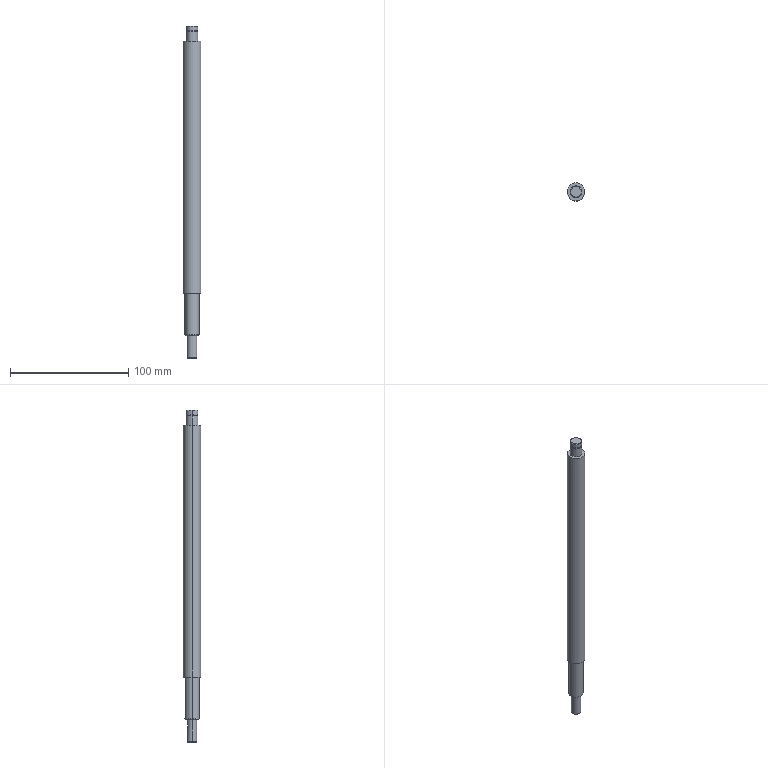Part | SolidWorks | features RevCut 4, Chamfer 2, Extrusion 1, ICE 1 | 1 solid | 28 faces | box 15 x 15 x 281 mm | volume 43646 mm3 | cylinder 12 | plane 9 | cone 7 | commonest cylinder face diameters 10 x4 8 x2 9.5 x2 12 x2 15 x2
STEP:
#1=CARTESIAN_POINT('',(4.5,0.,281.));
#2=VERTEX_POINT('',#1);
#3=CARTESIAN_POINT('',(-4.5,0.,281.));
#4=VERTEX_POINT('',#3);
#5=CARTESIAN_POINT('',(0.,0.,281.));
#6=DIRECTION('',(0.,0.,1.));
#7=DIRECTION('',(1.,0.,0.));
#8=AXIS2_PLACEMENT_3D('',#5,#6,#7);
#9=CIRCLE('',#8,4.5);
#10=EDGE_CURVE('',#2,#4,#9,.T.);
#11=ORIENTED_EDGE('',*,*,#10,.F.);
#12=CARTESIAN_POINT('',(5.,0.,280.5));
#13=VERTEX_POINT('',#12);
#14=CARTESIAN_POINT('',(4.5,0.,281.));
#15=DIRECTION('',(0.7071,0.,-0.7071));
#16=VECTOR('',#15,1000.);
#17=LINE('',#14,#16);
#18=EDGE_CURVE('',#2,#13,#17,.T.);
#19=ORIENTED_EDGE('',*,*,#18,.T.);
#20=CARTESIAN_POINT('',(-5.,0.,280.5));
#21=VERTEX_POINT('',#20);
#22=CARTESIAN_POINT('',(0.,0.,280.5));
#23=DIRECTION('',(0.,0.,-1.));
#24=DIRECTION('',(1.,0.,0.));
#25=AXIS2_PLACEMENT_3D('',#22,#23,#24);
#26=CIRCLE('',#25,5.);
#27=EDGE_CURVE('',#21,#13,#26,.T.);
#28=ORIENTED_EDGE('',*,*,#27,.F.);
#29=CARTESIAN_POINT('',(-4.5,0.,281.));
#30=DIRECTION('',(-0.7071,0.,-0.7071));
#31=VECTOR('',#30,1000.);
#32=LINE('',#29,#31);
#33=EDGE_CURVE('',#4,#21,#32,.T.);
#34=ORIENTED_EDGE('',*,*,#33,.F.);
#35=EDGE_LOOP('',(#11,#19,#28,#34));
#36=FACE_OUTER_BOUND('',#35,.T.);
#37=CARTESIAN_POINT('',(0.,0.,281.));
#38=DIRECTION('',(0.,0.,-1.));
#39=DIRECTION('',(-1.,0.,0.));
#40=AXIS2_PLACEMENT_3D('',#37,#38,#39);
#41=CONICAL_SURFACE('',#40,4.5,0.7854);
#42=ADVANCED_FACE('',(#36),#41,.T.);
#43=CARTESIAN_POINT('',(-5.,0.,277.1));
#44=VERTEX_POINT('',#43);
#45=CARTESIAN_POINT('',(5.,0.,277.1));
#46=VERTEX_POINT('',#45);
#47=CARTESIAN_POINT('',(0.,0.,277.1));
#48=DIRECTION('',(0.,0.,-1.));
#49=DIRECTION('',(1.,0.,0.));
#50=AXIS2_PLACEMENT_3D('',#47,#48,#49);
#51=CIRCLE('',#50,5.);
#52=EDGE_CURVE('',#44,#46,#51,.T.);
#53=ORIENTED_EDGE('',*,*,#52,.F.);
#54=CARTESIAN_POINT('',(-5.,0.,281.));
#55=DIRECTION('',(0.,0.,1.));
#56=VECTOR('',#55,1000.);
#57=LINE('',#54,#56);
#58=EDGE_CURVE('',#44,#21,#57,.T.);
#59=ORIENTED_EDGE('',*,*,#58,.T.);
#60=ORIENTED_EDGE('',*,*,#27,.T.);
#61=CARTESIAN_POINT('',(5.,0.,281.));
#62=DIRECTION('',(0.,0.,1.));
#63=VECTOR('',#62,1000.);
#64=LINE('',#61,#63);
#65=EDGE_CURVE('',#46,#13,#64,.T.);
#66=ORIENTED_EDGE('',*,*,#65,.F.);
#67=EDGE_LOOP('',(#53,#59,#60,#66));
#68=FACE_OUTER_BOUND('',#67,.T.);
#69=CARTESIAN_POINT('',(0.,0.,281.));
#70=DIRECTION('',(0.,0.,1.));
#71=DIRECTION('',(1.,0.,0.));
#72=AXIS2_PLACEMENT_3D('',#69,#70,#71);
#73=CYLINDRICAL_SURFACE('',#72,5.);
#74=ADVANCED_FACE('',(#68),#73,.T.);
#75=CARTESIAN_POINT('',(-4.75,0.,277.1));
#76=VERTEX_POINT('',#75);
#77=CARTESIAN_POINT('',(4.75,0.,277.1));
#78=VERTEX_POINT('',#77);
#79=CARTESIAN_POINT('',(0.,0.,277.1));
#80=DIRECTION('',(0.,0.,-1.));
#81=DIRECTION('',(-1.,0.,0.));
#82=AXIS2_PLACEMENT_3D('',#79,#80,#81);
#83=CIRCLE('',#82,4.75);
#84=EDGE_CURVE('',#76,#78,#83,.T.);
#85=ORIENTED_EDGE('',*,*,#84,.T.);
#86=CARTESIAN_POINT('',(4.75,0.,276.));
#87=VERTEX_POINT('',#86);
#88=CARTESIAN_POINT('',(4.75,0.,268.));
#89=DIRECTION('',(0.,0.,-1.));
#90=VECTOR('',#89,1000.);
#91=LINE('',#88,#90);
#92=EDGE_CURVE('',#78,#87,#91,.T.);
#93=ORIENTED_EDGE('',*,*,#92,.T.);
#94=CARTESIAN_POINT('',(-4.75,0.,276.));
#95=VERTEX_POINT('',#94);
#96=CARTESIAN_POINT('',(0.,0.,276.));
#97=DIRECTION('',(0.,0.,-1.));
#98=DIRECTION('',(-1.,0.,0.));
#99=AXIS2_PLACEMENT_3D('',#96,#97,#98);
#100=CIRCLE('',#99,4.75);
#101=EDGE_CURVE('',#95,#87,#100,.T.);
#102=ORIENTED_EDGE('',*,*,#101,.F.);
#103=CARTESIAN_POINT('',(-4.75,0.,268.));
#104=DIRECTION('',(0.,0.,-1.));
#105=VECTOR('',#104,1000.);
#106=LINE('',#103,#105);
#107=EDGE_CURVE('',#76,#95,#106,.T.);
#108=ORIENTED_EDGE('',*,*,#107,.F.);
#109=EDGE_LOOP('',(#85,#93,#102,#108));
#110=FACE_OUTER_BOUND('',#109,.T.);
#111=CARTESIAN_POINT('',(0.,0.,268.));
#112=DIRECTION('',(0.,0.,-1.));
#113=DIRECTION('',(-1.,0.,0.));
#114=AXIS2_PLACEMENT_3D('',#111,#112,#113);
#115=CYLINDRICAL_SURFACE('',#114,4.75);
#116=ADVANCED_FACE('',(#110),#115,.T.);
#117=CARTESIAN_POINT('',(-5.5,0.,19.));
#118=VERTEX_POINT('',#117);
#119=CARTESIAN_POINT('',(5.5,0.,19.));
#120=VERTEX_POINT('',#119);
#121=CARTESIAN_POINT('',(0.,0.,19.));
#122=DIRECTION('',(0.,0.,-1.));
#123=DIRECTION('',(1.,0.,0.));
#124=AXIS2_PLACEMENT_3D('',#121,#122,#123);
#125=CIRCLE('',#124,5.5);
#126=EDGE_CURVE('',#118,#120,#125,.T.);
#127=ORIENTED_EDGE('',*,*,#126,.F.);
#128=CARTESIAN_POINT('',(-6.,0.,19.5));
#129=VERTEX_POINT('',#128);
#130=CARTESIAN_POINT('',(-6.,0.,19.5));
#131=DIRECTION('',(-0.7071,0.,0.7071));
#132=VECTOR('',#131,1000.);
#133=LINE('',#130,#132);
#134=EDGE_CURVE('',#118,#129,#133,.T.);
#135=ORIENTED_EDGE('',*,*,#134,.T.);
#136=CARTESIAN_POINT('',(6.,0.,19.5));
#137=VERTEX_POINT('',#136);
#138=CARTESIAN_POINT('',(0.,0.,19.5));
#139=DIRECTION('',(0.,0.,1.));
#140=DIRECTION('',(1.,0.,0.));
#141=AXIS2_PLACEMENT_3D('',#138,#139,#140);
#142=CIRCLE('',#141,6.);
#143=EDGE_CURVE('',#137,#129,#142,.T.);
#144=ORIENTED_EDGE('',*,*,#143,.F.);
#145=CARTESIAN_POINT('',(6.,0.,19.5));
#146=DIRECTION('',(0.7071,0.,0.7071));
#147=VECTOR('',#146,1000.);
#148=LINE('',#145,#147);
#149=EDGE_CURVE('',#120,#137,#148,.T.);
#150=ORIENTED_EDGE('',*,*,#149,.F.);
#151=EDGE_LOOP('',(#127,#135,#144,#150));
#152=FACE_OUTER_BOUND('',#151,.T.);
#153=CARTESIAN_POINT('',(0.,0.,19.5));
#154=DIRECTION('',(0.,0.,1.));
#155=DIRECTION('',(1.,0.,0.));
#156=AXIS2_PLACEMENT_3D('',#153,#154,#155);
#157=CONICAL_SURFACE('',#156,6.,0.7854);
#158=ADVANCED_FACE('',(#152),#157,.T.);
#159=CARTESIAN_POINT('',(-3.5,0.,0.));
#160=VERTEX_POINT('',#159);
#161=CARTESIAN_POINT('',(0.,3.5,0.));
#162=VERTEX_POINT('',#161);
#163=CARTESIAN_POINT('',(0.,0.,0.));
#164=DIRECTION('',(0.,0.,-1.));
#165=DIRECTION('',(1.,0.,0.));
#166=AXIS2_PLACEMENT_3D('',#163,#164,#165);
#167=CIRCLE('',#166,3.5);
#168=EDGE_CURVE('',#160,#162,#167,.T.);
#169=ORIENTED_EDGE('',*,*,#168,.F.);
#170=CARTESIAN_POINT('',(-4.,0.,0.5));
#171=VERTEX_POINT('',#170);
#172=CARTESIAN_POINT('',(-3.5,0.,0.));
#173=DIRECTION('',(-0.7071,0.,0.7071));
#174=VECTOR('',#173,1000.);
#175=LINE('',#172,#174);
#176=EDGE_CURVE('',#160,#171,#175,.T.);
#177=ORIENTED_EDGE('',*,*,#176,.T.);
#178=CARTESIAN_POINT('',(-1.936,3.5,0.5));
#179=VERTEX_POINT('',#178);
#180=CARTESIAN_POINT('',(0.,0.,0.5));
#181=DIRECTION('',(0.,0.,1.));
#182=DIRECTION('',(1.,0.,0.));
#183=AXIS2_PLACEMENT_3D('',#180,#181,#182);
#184=CIRCLE('',#183,4.);
#185=EDGE_CURVE('',#179,#171,#184,.T.);
#186=ORIENTED_EDGE('',*,*,#185,.F.);
#187=CARTESIAN_POINT('',(0.,3.5,0.));
#188=CARTESIAN_POINT('',(-0.34,3.5,0.));
#189=CARTESIAN_POINT('',(-0.673,3.5,0.05018));
#190=CARTESIAN_POINT('',(-1.328,3.5,0.2302));
#191=CARTESIAN_POINT('',(-1.638,3.5,0.3555));
#192=CARTESIAN_POINT('',(-1.936,3.5,0.5));
#193=B_SPLINE_CURVE_WITH_KNOTS('',3,(#187,#188,#189,#190,#191,#192),.UNSPECIFIED.,.F.,.F.,(4,2,4),(0.004182,0.005183,0.006184),.UNSPECIFIED.);
#194=EDGE_CURVE('',#162,#179,#193,.T.);
#195=ORIENTED_EDGE('',*,*,#194,.F.);
#196=EDGE_LOOP('',(#169,#177,#186,#195));
#197=FACE_OUTER_BOUND('',#196,.T.);
#198=CARTESIAN_POINT('',(0.,0.,0.));
#199=DIRECTION('',(0.,0.,1.));
#200=DIRECTION('',(1.,0.,0.));
#201=AXIS2_PLACEMENT_3D('',#198,#199,#200);
#202=CONICAL_SURFACE('',#201,3.5,0.7854);
#203=ADVANCED_FACE('',(#197),#202,.T.);
#204=ORIENTED_EDGE('',*,*,#176,.F.);
#205=CARTESIAN_POINT('',(3.5,0.,0.));
#206=VERTEX_POINT('',#205);
#207=CARTESIAN_POINT('',(0.,0.,0.));
#208=DIRECTION('',(0.,0.,-1.));
#209=DIRECTION('',(1.,0.,0.));
#210=AXIS2_PLACEMENT_3D('',#207,#208,#209);
#211=CIRCLE('',#210,3.5);
#212=EDGE_CURVE('',#206,#160,#211,.T.);
#213=ORIENTED_EDGE('',*,*,#212,.F.);
#214=CARTESIAN_POINT('',(4.,0.,0.5));
#215=VERTEX_POINT('',#214);
#216=CARTESIAN_POINT('',(3.5,0.,0.));
#217=DIRECTION('',(0.7071,0.,0.7071));
#218=VECTOR('',#217,1000.);
#219=LINE('',#216,#218);
#220=EDGE_CURVE('',#206,#215,#219,.T.);
#221=ORIENTED_EDGE('',*,*,#220,.T.);
#222=CARTESIAN_POINT('',(0.,0.,0.5));
#223=DIRECTION('',(0.,0.,1.));
#224=DIRECTION('',(1.,0.,0.));
#225=AXIS2_PLACEMENT_3D('',#222,#223,#224);
#226=CIRCLE('',#225,4.);
#227=EDGE_CURVE('',#171,#215,#226,.T.);
#228=ORIENTED_EDGE('',*,*,#227,.F.);
#229=EDGE_LOOP('',(#204,#213,#221,#228));
#230=FACE_OUTER_BOUND('',#229,.T.);
#231=CARTESIAN_POINT('',(0.,0.,0.));
#232=DIRECTION('',(0.,0.,1.));
#233=DIRECTION('',(1.,0.,0.));
#234=AXIS2_PLACEMENT_3D('',#231,#232,#233);
#235=CONICAL_SURFACE('',#234,3.5,0.7854);
#236=ADVANCED_FACE('',(#230),#235,.T.);
#237=CARTESIAN_POINT('',(-4.,0.,19.));
#238=VERTEX_POINT('',#237);
#239=CARTESIAN_POINT('',(4.,0.,19.));
#240=VERTEX_POINT('',#239);
#241=CARTESIAN_POINT('',(0.,0.,19.));
#242=DIRECTION('',(0.,0.,-1.));
#243=DIRECTION('',(-1.,0.,0.));
#244=AXIS2_PLACEMENT_3D('',#241,#242,#243);
#245=CIRCLE('',#244,4.);
#246=EDGE_CURVE('',#238,#240,#245,.T.);
#247=ORIENTED_EDGE('',*,*,#246,.T.);
#248=CARTESIAN_POINT('',(4.,0.,0.));
#249=DIRECTION('',(0.,0.,-1.));
#250=VECTOR('',#249,1000.);
#251=LINE('',#248,#250);
#252=EDGE_CURVE('',#240,#215,#251,.T.);
#253=ORIENTED_EDGE('',*,*,#252,.T.);
#254=CARTESIAN_POINT('',(1.936,3.5,0.5));
#255=VERTEX_POINT('',#254);
#256=CARTESIAN_POINT('',(0.,0.,0.5));
#257=DIRECTION('',(0.,0.,1.));
#258=DIRECTION('',(1.,0.,0.));
#259=AXIS2_PLACEMENT_3D('',#256,#257,#258);
#260=CIRCLE('',#259,4.);
#261=EDGE_CURVE('',#215,#255,#260,.T.);
#262=ORIENTED_EDGE('',*,*,#261,.T.);
#263=CARTESIAN_POINT('',(1.936,3.5,17.));
#264=VERTEX_POINT('',#263);
#265=CARTESIAN_POINT('',(1.936,3.5,0.));
#266=DIRECTION('',(0.,0.,1.));
#267=VECTOR('',#266,1000.);
#268=LINE('',#265,#267);
#269=EDGE_CURVE('',#255,#264,#268,.T.);
#270=ORIENTED_EDGE('',*,*,#269,.T.);
#271=CARTESIAN_POINT('',(-1.936,3.5,17.));
#272=VERTEX_POINT('',#271);
#273=CARTESIAN_POINT('',(0.,0.,17.));
#274=DIRECTION('',(0.,0.,-1.));
#275=DIRECTION('',(-1.,0.,0.));
#276=AXIS2_PLACEMENT_3D('',#273,#274,#275);
#277=CIRCLE('',#276,4.);
#278=EDGE_CURVE('',#272,#264,#277,.T.);
#279=ORIENTED_EDGE('',*,*,#278,.F.);
#280=CARTESIAN_POINT('',(-1.936,3.5,0.));
#281=DIRECTION('',(0.,0.,-1.));
#282=VECTOR('',#281,1000.);
#283=LINE('',#280,#282);
#284=EDGE_CURVE('',#272,#179,#283,.T.);
#285=ORIENTED_EDGE('',*,*,#284,.T.);
#286=ORIENTED_EDGE('',*,*,#185,.T.);
#287=CARTESIAN_POINT('',(-4.,0.,0.));
#288=DIRECTION('',(0.,0.,-1.));
#289=VECTOR('',#288,1000.);
#290=LINE('',#287,#289);
#291=EDGE_CURVE('',#238,#171,#290,.T.);
#292=ORIENTED_EDGE('',*,*,#291,.F.);
#293=EDGE_LOOP('',(#247,#253,#262,#270,#279,#285,#286,#292));
#294=FACE_OUTER_BOUND('',#293,.T.);
#295=CARTESIAN_POINT('',(0.,0.,0.));
#296=DIRECTION('',(0.,0.,-1.));
#297=DIRECTION('',(-1.,0.,0.));
#298=AXIS2_PLACEMENT_3D('',#295,#296,#297);
#299=CYLINDRICAL_SURFACE('',#298,4.);
#300=ADVANCED_FACE('',(#294),#299,.T.);
#301=ORIENTED_EDGE('',*,*,#143,.T.);
#302=CARTESIAN_POINT('',(-6.,0.,55.));
#303=VERTEX_POINT('',#302);
#304=CARTESIAN_POINT('',(-6.,0.,268.));
#305=DIRECTION('',(0.,0.,1.));
#306=VECTOR('',#305,1000.);
#307=LINE('',#304,#306);
#308=EDGE_CURVE('',#129,#303,#307,.T.);
#309=ORIENTED_EDGE('',*,*,#308,.T.);
#310=CARTESIAN_POINT('',(6.,0.,55.));
#311=VERTEX_POINT('',#310);
#312=CARTESIAN_POINT('',(0.,0.,55.));
#313=DIRECTION('',(0.,0.,1.));
#314=DIRECTION('',(1.,0.,0.));
#315=AXIS2_PLACEMENT_3D('',#312,#313,#314);
#316=CIRCLE('',#315,6.);
#317=EDGE_CURVE('',#311,#303,#316,.T.);
#318=ORIENTED_EDGE('',*,*,#317,.F.);
#319=CARTESIAN_POINT('',(6.,0.,268.));
#320=DIRECTION('',(0.,0.,1.));
#321=VECTOR('',#320,1000.);
#322=LINE('',#319,#321);
#323=EDGE_CURVE('',#137,#311,#322,.T.);
#324=ORIENTED_EDGE('',*,*,#323,.F.);
#325=EDGE_LOOP('',(#301,#309,#318,#324));
#326=FACE_OUTER_BOUND('',#325,.T.);
#327=CARTESIAN_POINT('',(0.,0.,268.));
#328=DIRECTION('',(0.,0.,1.));
#329=DIRECTION('',(1.,0.,0.));
#330=AXIS2_PLACEMENT_3D('',#327,#328,#329);
#331=CYLINDRICAL_SURFACE('',#330,6.);
#332=ADVANCED_FACE('',(#326),#331,.T.);
#333=CARTESIAN_POINT('',(7.5,0.,268.));
#334=VERTEX_POINT('',#333);
#335=CARTESIAN_POINT('',(-7.5,0.,268.));
#336=VERTEX_POINT('',#335);
#337=CARTESIAN_POINT('',(0.,0.,268.));
#338=DIRECTION('',(0.,0.,1.));
#339=DIRECTION('',(1.,0.,0.));
#340=AXIS2_PLACEMENT_3D('',#337,#338,#339);
#341=CIRCLE('',#340,7.5);
#342=EDGE_CURVE('',#334,#336,#341,.T.);
#343=ORIENTED_EDGE('',*,*,#342,.F.);
#344=CARTESIAN_POINT('',(7.5,0.,55.));
#345=VERTEX_POINT('',#344);
#346=CARTESIAN_POINT('',(7.5,0.,281.));
#347=DIRECTION('',(0.,0.,-1.));
#348=VECTOR('',#347,1000.);
#349=LINE('',#346,#348);
#350=EDGE_CURVE('',#334,#345,#349,.T.);
#351=ORIENTED_EDGE('',*,*,#350,.T.);
#352=CARTESIAN_POINT('',(-7.5,0.,55.));
#353=VERTEX_POINT('',#352);
#354=CARTESIAN_POINT('',(0.,0.,55.));
#355=DIRECTION('',(0.,0.,1.));
#356=DIRECTION('',(1.,0.,0.));
#357=AXIS2_PLACEMENT_3D('',#354,#355,#356);
#358=CIRCLE('',#357,7.5);
#359=EDGE_CURVE('',#345,#353,#358,.T.);
#360=ORIENTED_EDGE('',*,*,#359,.T.);
#361=CARTESIAN_POINT('',(-7.5,0.,281.));
#362=DIRECTION('',(0.,0.,-1.));
#363=VECTOR('',#362,1000.);
#364=LINE('',#361,#363);
#365=EDGE_CURVE('',#336,#353,#364,.T.);
#366=ORIENTED_EDGE('',*,*,#365,.F.);
#367=EDGE_LOOP('',(#343,#351,#360,#366));
#368=FACE_OUTER_BOUND('',#367,.T.);
#369=CARTESIAN_POINT('',(0.,0.,281.));
#370=DIRECTION('',(0.,0.,-1.));
#371=DIRECTION('',(-1.,0.,0.));
#372=AXIS2_PLACEMENT_3D('',#369,#370,#371);
#373=CYLINDRICAL_SURFACE('',#372,7.5);
#374=ADVANCED_FACE('',(#368),#373,.T.);
#375=CARTESIAN_POINT('',(5.,0.,268.));
#376=VERTEX_POINT('',#375);
#377=CARTESIAN_POINT('',(-5.,0.,268.));
#378=VERTEX_POINT('',#377);
#379=CARTESIAN_POINT('',(0.,0.,268.));
#380=DIRECTION('',(0.,0.,1.));
#381=DIRECTION('',(1.,0.,0.));
#382=AXIS2_PLACEMENT_3D('',#379,#380,#381);
#383=CIRCLE('',#382,5.);
#384=EDGE_CURVE('',#376,#378,#383,.T.);
#385=ORIENTED_EDGE('',*,*,#384,.T.);
#386=CARTESIAN_POINT('',(-5.,0.,276.));
#387=VERTEX_POINT('',#386);
#388=CARTESIAN_POINT('',(-5.,0.,281.));
#389=DIRECTION('',(0.,0.,1.));
#390=VECTOR('',#389,1000.);
#391=LINE('',#388,#390);
#392=EDGE_CURVE('',#378,#387,#391,.T.);
#393=ORIENTED_EDGE('',*,*,#392,.T.);
#394=CARTESIAN_POINT('',(5.,0.,276.));
#395=VERTEX_POINT('',#394);
#396=CARTESIAN_POINT('',(0.,0.,276.));
#397=DIRECTION('',(0.,0.,1.));
#398=DIRECTION('',(-1.,0.,0.));
#399=AXIS2_PLACEMENT_3D('',#396,#397,#398);
#400=CIRCLE('',#399,5.);
#401=EDGE_CURVE('',#395,#387,#400,.T.);
#402=ORIENTED_EDGE('',*,*,#401,.F.);
#403=CARTESIAN_POINT('',(5.,0.,281.));
#404=DIRECTION('',(0.,0.,1.));
#405=VECTOR('',#404,1000.);
#406=LINE('',#403,#405);
#407=EDGE_CURVE('',#376,#395,#406,.T.);
#408=ORIENTED_EDGE('',*,*,#407,.F.);
#409=EDGE_LOOP('',(#385,#393,#402,#408));
#410=FACE_OUTER_BOUND('',#409,.T.);
#411=CARTESIAN_POINT('',(0.,0.,281.));
#412=DIRECTION('',(0.,0.,1.));
#413=DIRECTION('',(1.,0.,0.));
#414=AXIS2_PLACEMENT_3D('',#411,#412,#413);
#415=CYLINDRICAL_SURFACE('',#414,5.);
#416=ADVANCED_FACE('',(#410),#415,.T.);
#417=ORIENTED_EDGE('',*,*,#392,.F.);
#418=CARTESIAN_POINT('',(0.,0.,268.));
#419=DIRECTION('',(0.,0.,1.));
#420=DIRECTION('',(1.,0.,0.));
#421=AXIS2_PLACEMENT_3D('',#418,#419,#420);
#422=CIRCLE('',#421,5.);
#423=EDGE_CURVE('',#378,#376,#422,.T.);
#424=ORIENTED_EDGE('',*,*,#423,.T.);
#425=ORIENTED_EDGE('',*,*,#407,.T.);
#426=CARTESIAN_POINT('',(0.,0.,276.));
#427=DIRECTION('',(0.,0.,1.));
#428=DIRECTION('',(-1.,0.,0.));
#429=AXIS2_PLACEMENT_3D('',#426,#427,#428);
#430=CIRCLE('',#429,5.);
#431=EDGE_CURVE('',#387,#395,#430,.T.);
#432=ORIENTED_EDGE('',*,*,#431,.F.);
#433=EDGE_LOOP('',(#417,#424,#425,#432));
#434=FACE_OUTER_BOUND('',#433,.T.);
#435=CARTESIAN_POINT('',(0.,0.,281.));
#436=DIRECTION('',(0.,0.,1.));
#437=DIRECTION('',(1.,0.,0.));
#438=AXIS2_PLACEMENT_3D('',#435,#436,#437);
#439=CYLINDRICAL_SURFACE('',#438,5.);
#440=ADVANCED_FACE('',(#434),#439,.T.);
#441=ORIENTED_EDGE('',*,*,#350,.F.);
#442=CARTESIAN_POINT('',(0.,0.,268.));
#443=DIRECTION('',(0.,0.,1.));
#444=DIRECTION('',(1.,0.,0.));
#445=AXIS2_PLACEMENT_3D('',#442,#443,#444);
#446=CIRCLE('',#445,7.5);
#447=EDGE_CURVE('',#336,#334,#446,.T.);
#448=ORIENTED_EDGE('',*,*,#447,.F.);
#449=ORIENTED_EDGE('',*,*,#365,.T.);
#450=CARTESIAN_POINT('',(0.,0.,55.));
#451=DIRECTION('',(0.,0.,1.));
#452=DIRECTION('',(1.,0.,0.));
#453=AXIS2_PLACEMENT_3D('',#450,#451,#452);
#454=CIRCLE('',#453,7.5);
#455=EDGE_CURVE('',#353,#345,#454,.T.);
#456=ORIENTED_EDGE('',*,*,#455,.T.);
#457=EDGE_LOOP('',(#441,#448,#449,#456));
#458=FACE_OUTER_BOUND('',#457,.T.);
#459=CARTESIAN_POINT('',(0.,0.,281.));
#460=DIRECTION('',(0.,0.,-1.));
#461=DIRECTION('',(-1.,0.,0.));
#462=AXIS2_PLACEMENT_3D('',#459,#460,#461);
#463=CYLINDRICAL_SURFACE('',#462,7.5);
#464=ADVANCED_FACE('',(#458),#463,.T.);
#465=ORIENTED_EDGE('',*,*,#384,.F.);
#466=ORIENTED_EDGE('',*,*,#423,.F.);
#467=EDGE_LOOP('',(#465,#466));
#468=FACE_BOUND('',#467,.T.);
#469=ORIENTED_EDGE('',*,*,#447,.T.);
#470=ORIENTED_EDGE('',*,*,#342,.T.);
#471=EDGE_LOOP('',(#469,#470));
#472=FACE_OUTER_BOUND('',#471,.T.);
#473=CARTESIAN_POINT('',(-53.874,0.,268.));
#474=DIRECTION('',(0.,0.,1.));
#475=DIRECTION('',(1.,0.,0.));
#476=AXIS2_PLACEMENT_3D('',#473,#474,#475);
#477=PLANE('',#476);
#478=ADVANCED_FACE('',(#468,#472),#477,.T.);
#479=ORIENTED_EDGE('',*,*,#317,.T.);
#480=CARTESIAN_POINT('',(0.,0.,55.));
#481=DIRECTION('',(0.,0.,1.));
#482=DIRECTION('',(1.,0.,0.));
#483=AXIS2_PLACEMENT_3D('',#480,#481,#482);
#484=CIRCLE('',#483,6.);
#485=EDGE_CURVE('',#303,#311,#484,.T.);
#486=ORIENTED_EDGE('',*,*,#485,.T.);
#487=EDGE_LOOP('',(#479,#486));
#488=FACE_BOUND('',#487,.T.);
#489=ORIENTED_EDGE('',*,*,#455,.F.);
#490=ORIENTED_EDGE('',*,*,#359,.F.);
#491=EDGE_LOOP('',(#489,#490));
#492=FACE_OUTER_BOUND('',#491,.T.);
#493=CARTESIAN_POINT('',(41.836,0.,55.));
#494=DIRECTION('',(0.,0.,1.));
#495=DIRECTION('',(1.,0.,0.));
#496=AXIS2_PLACEMENT_3D('',#493,#494,#495);
#497=PLANE('',#496);
#498=ADVANCED_FACE('',(#488,#492),#497,.F.);
#499=ORIENTED_EDGE('',*,*,#308,.F.);
#500=CARTESIAN_POINT('',(0.,0.,19.5));
#501=DIRECTION('',(0.,0.,1.));
#502=DIRECTION('',(1.,0.,0.));
#503=AXIS2_PLACEMENT_3D('',#500,#501,#502);
#504=CIRCLE('',#503,6.);
#505=EDGE_CURVE('',#129,#137,#504,.T.);
#506=ORIENTED_EDGE('',*,*,#505,.T.);
#507=ORIENTED_EDGE('',*,*,#323,.T.);
#508=ORIENTED_EDGE('',*,*,#485,.F.);
#509=EDGE_LOOP('',(#499,#506,#507,#508));
#510=FACE_OUTER_BOUND('',#509,.T.);
#511=CARTESIAN_POINT('',(0.,0.,268.));
#512=DIRECTION('',(0.,0.,1.));
#513=DIRECTION('',(1.,0.,0.));
#514=AXIS2_PLACEMENT_3D('',#511,#512,#513);
#515=CYLINDRICAL_SURFACE('',#514,6.);
#516=ADVANCED_FACE('',(#510),#515,.T.);
#517=CARTESIAN_POINT('',(0.,0.,19.));
#518=DIRECTION('',(0.,0.,-1.));
#519=DIRECTION('',(1.,0.,0.));
#520=AXIS2_PLACEMENT_3D('',#517,#518,#519);
#521=CIRCLE('',#520,5.5);
#522=EDGE_CURVE('',#120,#118,#521,.T.);
#523=ORIENTED_EDGE('',*,*,#522,.T.);
#524=ORIENTED_EDGE('',*,*,#126,.T.);
#525=EDGE_LOOP('',(#523,#524));
#526=FACE_OUTER_BOUND('',#525,.T.);
#527=ORIENTED_EDGE('',*,*,#246,.F.);
#528=CARTESIAN_POINT('',(0.,0.,19.));
#529=DIRECTION('',(0.,0.,-1.));
#530=DIRECTION('',(-1.,0.,0.));
#531=AXIS2_PLACEMENT_3D('',#528,#529,#530);
#532=CIRCLE('',#531,4.);
#533=EDGE_CURVE('',#240,#238,#532,.T.);
#534=ORIENTED_EDGE('',*,*,#533,.F.);
#535=EDGE_LOOP('',(#527,#534));
#536=FACE_BOUND('',#535,.T.);
#537=CARTESIAN_POINT('',(-37.149,0.,19.));
#538=DIRECTION('',(0.,0.,1.));
#539=DIRECTION('',(1.,0.,0.));
#540=AXIS2_PLACEMENT_3D('',#537,#538,#539);
#541=PLANE('',#540);
#542=ADVANCED_FACE('',(#526,#536),#541,.F.);
#543=ORIENTED_EDGE('',*,*,#252,.F.);
#544=ORIENTED_EDGE('',*,*,#533,.T.);
#545=ORIENTED_EDGE('',*,*,#291,.T.);
#546=ORIENTED_EDGE('',*,*,#227,.T.);
#547=EDGE_LOOP('',(#543,#544,#545,#546));
#548=FACE_OUTER_BOUND('',#547,.T.);
#549=CARTESIAN_POINT('',(0.,0.,0.));
#550=DIRECTION('',(0.,0.,-1.));
#551=DIRECTION('',(-1.,0.,0.));
#552=AXIS2_PLACEMENT_3D('',#549,#550,#551);
#553=CYLINDRICAL_SURFACE('',#552,4.);
#554=ADVANCED_FACE('',(#548),#553,.T.);
#555=CARTESIAN_POINT('',(0.,0.,0.));
#556=DIRECTION('',(0.,0.,-1.));
#557=DIRECTION('',(1.,0.,0.));
#558=AXIS2_PLACEMENT_3D('',#555,#556,#557);
#559=CIRCLE('',#558,3.5);
#560=EDGE_CURVE('',#162,#206,#559,.T.);
#561=ORIENTED_EDGE('',*,*,#560,.T.);
#562=ORIENTED_EDGE('',*,*,#212,.T.);
#563=ORIENTED_EDGE('',*,*,#168,.T.);
#564=EDGE_LOOP('',(#561,#562,#563));
#565=FACE_OUTER_BOUND('',#564,.T.);
#566=CARTESIAN_POINT('',(0.,0.,0.));
#567=DIRECTION('',(0.,0.,1.));
#568=DIRECTION('',(1.,0.,0.));
#569=AXIS2_PLACEMENT_3D('',#566,#567,#568);
#570=PLANE('',#569);
#571=ADVANCED_FACE('',(#565),#570,.F.);
#572=ORIENTED_EDGE('',*,*,#220,.F.);
#573=ORIENTED_EDGE('',*,*,#560,.F.);
#574=CARTESIAN_POINT('',(1.936,3.5,0.5));
#575=CARTESIAN_POINT('',(1.786,3.5,0.4273));
#576=CARTESIAN_POINT('',(1.633,3.5,0.3596));
#577=CARTESIAN_POINT('',(1.319,3.5,0.2376));
#578=CARTESIAN_POINT('',(1.158,3.5,0.1834));
#579=CARTESIAN_POINT('',(0.6719,3.5,0.05023));
#580=CARTESIAN_POINT('',(0.3393,3.5,0.));
#581=CARTESIAN_POINT('',(0.,3.5,0.));
#582=B_SPLINE_CURVE_WITH_KNOTS('',3,(#574,#575,#576,#577,#578,#579,#580,#581),.UNSPECIFIED.,.F.,.F.,(4,2,2,4),(0.002184,0.002684,0.003183,0.004182),.UNSPECIFIED.);
#583=EDGE_CURVE('',#255,#162,#582,.T.);
#584=ORIENTED_EDGE('',*,*,#583,.F.);
#585=ORIENTED_EDGE('',*,*,#261,.F.);
#586=EDGE_LOOP('',(#572,#573,#584,#585));
#587=FACE_OUTER_BOUND('',#586,.T.);
#588=CARTESIAN_POINT('',(0.,0.,0.));
#589=DIRECTION('',(0.,0.,1.));
#590=DIRECTION('',(1.,0.,0.));
#591=AXIS2_PLACEMENT_3D('',#588,#589,#590);
#592=CONICAL_SURFACE('',#591,3.5,0.7854);
#593=ADVANCED_FACE('',(#587),#592,.T.);
#594=ORIENTED_EDGE('',*,*,#134,.F.);
#595=ORIENTED_EDGE('',*,*,#522,.F.);
#596=ORIENTED_EDGE('',*,*,#149,.T.);
#597=ORIENTED_EDGE('',*,*,#505,.F.);
#598=EDGE_LOOP('',(#594,#595,#596,#597));
#599=FACE_OUTER_BOUND('',#598,.T.);
#600=CARTESIAN_POINT('',(0.,0.,19.5));
#601=DIRECTION('',(0.,0.,1.));
#602=DIRECTION('',(1.,0.,0.));
#603=AXIS2_PLACEMENT_3D('',#600,#601,#602);
#604=CONICAL_SURFACE('',#603,6.,0.7854);
#605=ADVANCED_FACE('',(#599),#604,.T.);
#606=ORIENTED_EDGE('',*,*,#92,.F.);
#607=CARTESIAN_POINT('',(0.,0.,277.1));
#608=DIRECTION('',(0.,0.,-1.));
#609=DIRECTION('',(-1.,0.,0.));
#610=AXIS2_PLACEMENT_3D('',#607,#608,#609);
#611=CIRCLE('',#610,4.75);
#612=EDGE_CURVE('',#78,#76,#611,.T.);
#613=ORIENTED_EDGE('',*,*,#612,.T.);
#614=ORIENTED_EDGE('',*,*,#107,.T.);
#615=CARTESIAN_POINT('',(0.,0.,276.));
#616=DIRECTION('',(0.,0.,-1.));
#617=DIRECTION('',(-1.,0.,0.));
#618=AXIS2_PLACEMENT_3D('',#615,#616,#617);
#619=CIRCLE('',#618,4.75);
#620=EDGE_CURVE('',#87,#95,#619,.T.);
#621=ORIENTED_EDGE('',*,*,#620,.F.);
#622=EDGE_LOOP('',(#606,#613,#614,#621));
#623=FACE_OUTER_BOUND('',#622,.T.);
#624=CARTESIAN_POINT('',(0.,0.,268.));
#625=DIRECTION('',(0.,0.,-1.));
#626=DIRECTION('',(-1.,0.,0.));
#627=AXIS2_PLACEMENT_3D('',#624,#625,#626);
#628=CYLINDRICAL_SURFACE('',#627,4.75);
#629=ADVANCED_FACE('',(#623),#628,.T.);
#630=ORIENTED_EDGE('',*,*,#401,.T.);
#631=ORIENTED_EDGE('',*,*,#431,.T.);
#632=EDGE_LOOP('',(#630,#631));
#633=FACE_OUTER_BOUND('',#632,.T.);
#634=ORIENTED_EDGE('',*,*,#101,.T.);
#635=ORIENTED_EDGE('',*,*,#620,.T.);
#636=EDGE_LOOP('',(#634,#635));
#637=FACE_BOUND('',#636,.T.);
#638=CARTESIAN_POINT('',(-20.041,0.,276.));
#639=DIRECTION('',(0.,0.,-1.));
#640=DIRECTION('',(-1.,0.,0.));
#641=AXIS2_PLACEMENT_3D('',#638,#639,#640);
#642=PLANE('',#641);
#643=ADVANCED_FACE('',(#633,#637),#642,.F.);
#644=CARTESIAN_POINT('',(0.,0.,277.1));
#645=DIRECTION('',(0.,0.,-1.));
#646=DIRECTION('',(1.,0.,0.));
#647=AXIS2_PLACEMENT_3D('',#644,#645,#646);
#648=CIRCLE('',#647,5.);
#649=EDGE_CURVE('',#46,#44,#648,.T.);
#650=ORIENTED_EDGE('',*,*,#649,.T.);
#651=ORIENTED_EDGE('',*,*,#52,.T.);
#652=EDGE_LOOP('',(#650,#651));
#653=FACE_OUTER_BOUND('',#652,.T.);
#654=ORIENTED_EDGE('',*,*,#84,.F.);
#655=ORIENTED_EDGE('',*,*,#612,.F.);
#656=EDGE_LOOP('',(#654,#655));
#657=FACE_BOUND('',#656,.T.);
#658=CARTESIAN_POINT('',(-20.041,0.,277.1));
#659=DIRECTION('',(0.,0.,1.));
#660=DIRECTION('',(1.,0.,0.));
#661=AXIS2_PLACEMENT_3D('',#658,#659,#660);
#662=PLANE('',#661);
#663=ADVANCED_FACE('',(#653,#657),#662,.F.);
#664=CARTESIAN_POINT('',(0.,0.,281.));
#665=DIRECTION('',(0.,0.,1.));
#666=DIRECTION('',(1.,0.,0.));
#667=AXIS2_PLACEMENT_3D('',#664,#665,#666);
#668=CIRCLE('',#667,4.5);
#669=EDGE_CURVE('',#4,#2,#668,.T.);
#670=ORIENTED_EDGE('',*,*,#669,.T.);
#671=ORIENTED_EDGE('',*,*,#10,.T.);
#672=EDGE_LOOP('',(#670,#671));
#673=FACE_OUTER_BOUND('',#672,.T.);
#674=CARTESIAN_POINT('',(0.,0.,281.));
#675=DIRECTION('',(0.,0.,1.));
#676=DIRECTION('',(1.,0.,0.));
#677=AXIS2_PLACEMENT_3D('',#674,#675,#676);
#678=PLANE('',#677);
#679=ADVANCED_FACE('',(#673),#678,.T.);
#680=ORIENTED_EDGE('',*,*,#58,.F.);
#681=ORIENTED_EDGE('',*,*,#649,.F.);
#682=ORIENTED_EDGE('',*,*,#65,.T.);
#683=CARTESIAN_POINT('',(0.,0.,280.5));
#684=DIRECTION('',(0.,0.,-1.));
#685=DIRECTION('',(1.,0.,0.));
#686=AXIS2_PLACEMENT_3D('',#683,#684,#685);
#687=CIRCLE('',#686,5.);
#688=EDGE_CURVE('',#13,#21,#687,.T.);
#689=ORIENTED_EDGE('',*,*,#688,.T.);
#690=EDGE_LOOP('',(#680,#681,#682,#689));
#691=FACE_OUTER_BOUND('',#690,.T.);
#692=CARTESIAN_POINT('',(0.,0.,281.));
#693=DIRECTION('',(0.,0.,1.));
#694=DIRECTION('',(1.,0.,0.));
#695=AXIS2_PLACEMENT_3D('',#692,#693,#694);
#696=CYLINDRICAL_SURFACE('',#695,5.);
#697=ADVANCED_FACE('',(#691),#696,.T.);
#698=ORIENTED_EDGE('',*,*,#18,.F.);
#699=ORIENTED_EDGE('',*,*,#669,.F.);
#700=ORIENTED_EDGE('',*,*,#33,.T.);
#701=ORIENTED_EDGE('',*,*,#688,.F.);
#702=EDGE_LOOP('',(#698,#699,#700,#701));
#703=FACE_OUTER_BOUND('',#702,.T.);
#704=CARTESIAN_POINT('',(0.,0.,281.));
#705=DIRECTION('',(0.,0.,-1.));
#706=DIRECTION('',(-1.,0.,0.));
#707=AXIS2_PLACEMENT_3D('',#704,#705,#706);
#708=CONICAL_SURFACE('',#707,4.5,0.7854);
#709=ADVANCED_FACE('',(#703),#708,.T.);
#710=ORIENTED_EDGE('',*,*,#278,.T.);
#711=CARTESIAN_POINT('',(18.031,3.5,17.));
#712=DIRECTION('',(-1.,0.,0.));
#713=VECTOR('',#712,1000.);
#714=LINE('',#711,#713);
#715=EDGE_CURVE('',#264,#272,#714,.T.);
#716=ORIENTED_EDGE('',*,*,#715,.T.);
#717=EDGE_LOOP('',(#710,#716));
#718=FACE_OUTER_BOUND('',#717,.T.);
#719=CARTESIAN_POINT('',(0.,0.,17.));
#720=DIRECTION('',(0.,0.,-1.));
#721=DIRECTION('',(-1.,0.,0.));
#722=AXIS2_PLACEMENT_3D('',#719,#720,#721);
#723=PLANE('',#722);
#724=ADVANCED_FACE('',(#718),#723,.T.);
#725=ORIENTED_EDGE('',*,*,#715,.F.);
#726=ORIENTED_EDGE('',*,*,#269,.F.);
#727=ORIENTED_EDGE('',*,*,#583,.T.);
#728=ORIENTED_EDGE('',*,*,#194,.T.);
#729=ORIENTED_EDGE('',*,*,#284,.F.);
#730=EDGE_LOOP('',(#725,#726,#727,#728,#729));
#731=FACE_OUTER_BOUND('',#730,.T.);
#732=CARTESIAN_POINT('',(18.031,3.5,17.));
#733=DIRECTION('',(0.,-1.,0.));
#734=DIRECTION('',(1.,0.,0.));
#735=AXIS2_PLACEMENT_3D('',#732,#733,#734);
#736=PLANE('',#735);
#737=ADVANCED_FACE('',(#731),#736,.F.);
#738=CLOSED_SHELL('',(#42,#74,#116,#158,#203,#236,#300,#332,#374,#416,#440,#464,#478,#498,#516,#542,#554,#571,#593,#605,#629,#643,#663,#679,#697,#709,#724,#737));
#739=MANIFOLD_SOLID_BREP('',#738);
#740=CARTESIAN_POINT('',(0.,0.,0.));
#741=DIRECTION('',(0.,0.,1.));
#742=DIRECTION('',(1.,0.,0.));
#743=AXIS2_PLACEMENT_3D('',#740,#741,#742);
#744=(LENGTH_UNIT()NAMED_UNIT(*)SI_UNIT(.MILLI.,.METRE.));
#745=UNCERTAINTY_MEASURE_WITH_UNIT(LENGTH_MEASURE(0.00001),#744,'','');
#746=(NAMED_UNIT(*)PLANE_ANGLE_UNIT()SI_UNIT($,.RADIAN.));
#747=(NAMED_UNIT(*)SI_UNIT($,.STERADIAN.)SOLID_ANGLE_UNIT());
#748=(GEOMETRIC_REPRESENTATION_CONTEXT(3)GLOBAL_UNCERTAINTY_ASSIGNED_CONTEXT((#745))GLOBAL_UNIT_ASSIGNED_CONTEXT((#744,#746,#747))REPRESENTATION_CONTEXT('',''));
#749=ADVANCED_BREP_SHAPE_REPRESENTATION('',(#739,#743),#748);